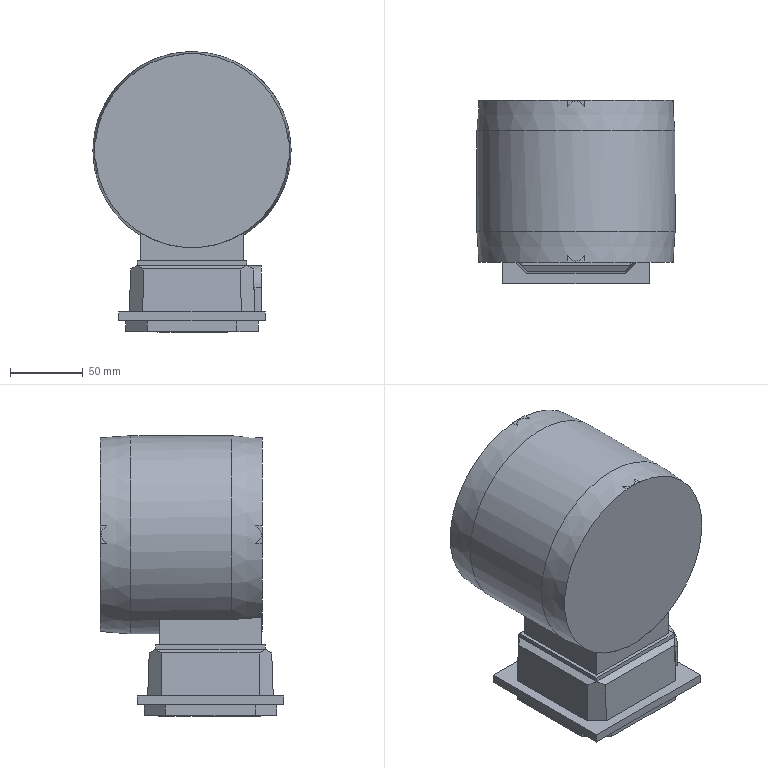Part | STEP file | 1 | 1 solid | 243 faces | box 135.85 x 125.7 x 192.425 mm | volume 2018687 mm3 | cylinder 128 | plane 113 | cone 2 | commonest cylinder face diameters 24.804 x20 83.121 x20 33.098 x10 46.586 x10 20 x2 30 x2